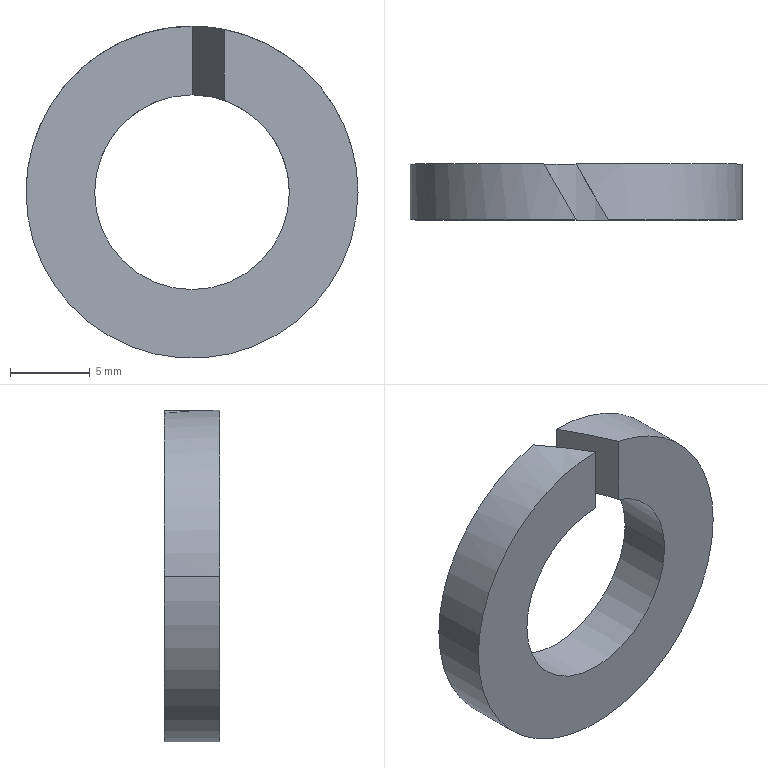Part | SolidWorks | features BaseBody 1 | 1 solid | 10 faces | box 20.8 x 3.5 x 20.8 mm | volume 749.557 mm3 | cylinder 6 | plane 4 | commonest cylinder face diameters 12.2 x3 20.8 x3
STEP:
#1=CARTESIAN_POINT('',(215.5,175.2,30.35));
#2=VERTEX_POINT('',#1);
#3=CARTESIAN_POINT('',(209.4,175.2,24.25));
#4=VERTEX_POINT('',#3);
#5=CARTESIAN_POINT('',(215.5,175.2,24.25));
#6=DIRECTION('',(0.,-1.,0.));
#7=DIRECTION('',(1.,0.,0.));
#8=AXIS2_PLACEMENT_3D('',#5,#6,#7);
#9=CIRCLE('',#8,6.1);
#10=EDGE_CURVE('',#2,#4,#9,.T.);
#11=ORIENTED_EDGE('',*,*,#10,.T.);
#12=CARTESIAN_POINT('',(209.4,178.7,24.25));
#13=VERTEX_POINT('',#12);
#14=CARTESIAN_POINT('',(209.4,175.2,24.25));
#15=DIRECTION('',(0.,1.,0.));
#16=VECTOR('',#15,1000.);
#17=LINE('',#14,#16);
#18=EDGE_CURVE('',#4,#13,#17,.T.);
#19=ORIENTED_EDGE('',*,*,#18,.T.);
#20=CARTESIAN_POINT('',(213.479,178.7,30.006));
#21=VERTEX_POINT('',#20);
#22=CARTESIAN_POINT('',(215.5,178.7,24.25));
#23=DIRECTION('',(0.,-1.,0.));
#24=DIRECTION('',(-1.,0.,0.));
#25=AXIS2_PLACEMENT_3D('',#22,#23,#24);
#26=CIRCLE('',#25,6.1);
#27=EDGE_CURVE('',#21,#13,#26,.T.);
#28=ORIENTED_EDGE('',*,*,#27,.F.);
#29=CARTESIAN_POINT('',(215.5,175.2,30.35));
#30=CARTESIAN_POINT('',(214.81,176.395,30.35));
#31=CARTESIAN_POINT('',(214.13,177.573,30.234));
#32=CARTESIAN_POINT('',(213.479,178.7,30.006));
#33=(BOUNDED_CURVE()B_SPLINE_CURVE(3,(#29,#30,#31,#32),.UNSPECIFIED.,.F.,.F.)B_SPLINE_CURVE_WITH_KNOTS((4,4),(4.712,5.05),.UNSPECIFIED.)CURVE()GEOMETRIC_REPRESENTATION_ITEM()RATIONAL_B_SPLINE_CURVE((1.,0.9905,0.9905,1.))REPRESENTATION_ITEM(''));
#34=EDGE_CURVE('',#2,#21,#33,.T.);
#35=ORIENTED_EDGE('',*,*,#34,.F.);
#36=EDGE_LOOP('',(#11,#19,#28,#35));
#37=FACE_OUTER_BOUND('',#36,.T.);
#38=CARTESIAN_POINT('',(215.5,175.2,24.25));
#39=DIRECTION('',(0.,1.,0.));
#40=DIRECTION('',(1.,0.,0.));
#41=AXIS2_PLACEMENT_3D('',#38,#39,#40);
#42=CYLINDRICAL_SURFACE('',#41,6.1);
#43=ADVANCED_FACE('',(#37),#42,.F.);
#44=ORIENTED_EDGE('',*,*,#18,.F.);
#45=CARTESIAN_POINT('',(221.6,175.2,24.25));
#46=VERTEX_POINT('',#45);
#47=CARTESIAN_POINT('',(215.5,175.2,24.25));
#48=DIRECTION('',(0.,-1.,0.));
#49=DIRECTION('',(1.,0.,0.));
#50=AXIS2_PLACEMENT_3D('',#47,#48,#49);
#51=CIRCLE('',#50,6.1);
#52=EDGE_CURVE('',#4,#46,#51,.T.);
#53=ORIENTED_EDGE('',*,*,#52,.T.);
#54=CARTESIAN_POINT('',(221.6,178.7,24.25));
#55=VERTEX_POINT('',#54);
#56=CARTESIAN_POINT('',(221.6,175.2,24.25));
#57=DIRECTION('',(0.,1.,0.));
#58=VECTOR('',#57,1000.);
#59=LINE('',#56,#58);
#60=EDGE_CURVE('',#46,#55,#59,.T.);
#61=ORIENTED_EDGE('',*,*,#60,.T.);
#62=CARTESIAN_POINT('',(215.5,178.7,24.25));
#63=DIRECTION('',(0.,-1.,0.));
#64=DIRECTION('',(-1.,0.,0.));
#65=AXIS2_PLACEMENT_3D('',#62,#63,#64);
#66=CIRCLE('',#65,6.1);
#67=EDGE_CURVE('',#13,#55,#66,.T.);
#68=ORIENTED_EDGE('',*,*,#67,.F.);
#69=EDGE_LOOP('',(#44,#53,#61,#68));
#70=FACE_OUTER_BOUND('',#69,.T.);
#71=CARTESIAN_POINT('',(215.5,175.2,24.25));
#72=DIRECTION('',(0.,1.,0.));
#73=DIRECTION('',(1.,0.,0.));
#74=AXIS2_PLACEMENT_3D('',#71,#72,#73);
#75=CYLINDRICAL_SURFACE('',#74,6.1);
#76=ADVANCED_FACE('',(#70),#75,.F.);
#77=CARTESIAN_POINT('',(205.1,175.2,24.25));
#78=VERTEX_POINT('',#77);
#79=CARTESIAN_POINT('',(225.9,175.2,24.25));
#80=VERTEX_POINT('',#79);
#81=CARTESIAN_POINT('',(215.5,175.2,24.25));
#82=DIRECTION('',(0.,-1.,0.));
#83=DIRECTION('',(1.,0.,0.));
#84=AXIS2_PLACEMENT_3D('',#81,#82,#83);
#85=CIRCLE('',#84,10.4);
#86=EDGE_CURVE('',#78,#80,#85,.T.);
#87=ORIENTED_EDGE('',*,*,#86,.F.);
#88=CARTESIAN_POINT('',(205.1,178.7,24.25));
#89=VERTEX_POINT('',#88);
#90=CARTESIAN_POINT('',(205.1,175.2,24.25));
#91=DIRECTION('',(0.,1.,0.));
#92=VECTOR('',#91,1000.);
#93=LINE('',#90,#92);
#94=EDGE_CURVE('',#78,#89,#93,.T.);
#95=ORIENTED_EDGE('',*,*,#94,.T.);
#96=CARTESIAN_POINT('',(225.9,178.7,24.25));
#97=VERTEX_POINT('',#96);
#98=CARTESIAN_POINT('',(215.5,178.7,24.25));
#99=DIRECTION('',(0.,-1.,0.));
#100=DIRECTION('',(-1.,0.,0.));
#101=AXIS2_PLACEMENT_3D('',#98,#99,#100);
#102=CIRCLE('',#101,10.4);
#103=EDGE_CURVE('',#89,#97,#102,.T.);
#104=ORIENTED_EDGE('',*,*,#103,.T.);
#105=CARTESIAN_POINT('',(225.9,175.2,24.25));
#106=DIRECTION('',(0.,1.,0.));
#107=VECTOR('',#106,1000.);
#108=LINE('',#105,#107);
#109=EDGE_CURVE('',#80,#97,#108,.T.);
#110=ORIENTED_EDGE('',*,*,#109,.F.);
#111=EDGE_LOOP('',(#87,#95,#104,#110));
#112=FACE_OUTER_BOUND('',#111,.T.);
#113=CARTESIAN_POINT('',(215.5,175.2,24.25));
#114=DIRECTION('',(0.,1.,0.));
#115=DIRECTION('',(1.,0.,0.));
#116=AXIS2_PLACEMENT_3D('',#113,#114,#115);
#117=CYLINDRICAL_SURFACE('',#116,10.4);
#118=ADVANCED_FACE('',(#112),#117,.T.);
#119=CARTESIAN_POINT('',(217.521,175.2,34.452));
#120=VERTEX_POINT('',#119);
#121=CARTESIAN_POINT('',(215.5,175.2,24.25));
#122=DIRECTION('',(0.,-1.,0.));
#123=DIRECTION('',(1.,0.,0.));
#124=AXIS2_PLACEMENT_3D('',#121,#122,#123);
#125=CIRCLE('',#124,10.4);
#126=EDGE_CURVE('',#80,#120,#125,.T.);
#127=ORIENTED_EDGE('',*,*,#126,.F.);
#128=ORIENTED_EDGE('',*,*,#109,.T.);
#129=CARTESIAN_POINT('',(215.5,178.7,34.65));
#130=VERTEX_POINT('',#129);
#131=CARTESIAN_POINT('',(215.5,178.7,24.25));
#132=DIRECTION('',(0.,-1.,0.));
#133=DIRECTION('',(-1.,0.,0.));
#134=AXIS2_PLACEMENT_3D('',#131,#132,#133);
#135=CIRCLE('',#134,10.4);
#136=EDGE_CURVE('',#97,#130,#135,.T.);
#137=ORIENTED_EDGE('',*,*,#136,.T.);
#138=CARTESIAN_POINT('',(215.5,178.7,34.65));
#139=CARTESIAN_POINT('',(216.179,177.524,34.65));
#140=CARTESIAN_POINT('',(216.855,176.354,34.584));
#141=CARTESIAN_POINT('',(217.521,175.2,34.452));
#142=(BOUNDED_CURVE()B_SPLINE_CURVE(3,(#138,#139,#140,#141),.UNSPECIFIED.,.F.,.F.)B_SPLINE_CURVE_WITH_KNOTS((4,4),(1.571,1.766),.UNSPECIFIED.)CURVE()GEOMETRIC_REPRESENTATION_ITEM()RATIONAL_B_SPLINE_CURVE((1.,0.9968,0.9968,1.))REPRESENTATION_ITEM(''));
#143=EDGE_CURVE('',#130,#120,#142,.T.);
#144=ORIENTED_EDGE('',*,*,#143,.T.);
#145=EDGE_LOOP('',(#127,#128,#137,#144));
#146=FACE_OUTER_BOUND('',#145,.T.);
#147=CARTESIAN_POINT('',(215.5,175.2,24.25));
#148=DIRECTION('',(0.,1.,0.));
#149=DIRECTION('',(1.,0.,0.));
#150=AXIS2_PLACEMENT_3D('',#147,#148,#149);
#151=CYLINDRICAL_SURFACE('',#150,10.4);
#152=ADVANCED_FACE('',(#146),#151,.T.);
#153=ORIENTED_EDGE('',*,*,#10,.F.);
#154=CARTESIAN_POINT('',(215.5,175.2,34.65));
#155=VERTEX_POINT('',#154);
#156=CARTESIAN_POINT('',(215.5,175.2,34.65));
#157=DIRECTION('',(0.,0.,-1.));
#158=VECTOR('',#157,1000.);
#159=LINE('',#156,#158);
#160=EDGE_CURVE('',#155,#2,#159,.T.);
#161=ORIENTED_EDGE('',*,*,#160,.F.);
#162=CARTESIAN_POINT('',(215.5,175.2,24.25));
#163=DIRECTION('',(0.,-1.,0.));
#164=DIRECTION('',(1.,0.,0.));
#165=AXIS2_PLACEMENT_3D('',#162,#163,#164);
#166=CIRCLE('',#165,10.4);
#167=EDGE_CURVE('',#155,#78,#166,.T.);
#168=ORIENTED_EDGE('',*,*,#167,.T.);
#169=ORIENTED_EDGE('',*,*,#86,.T.);
#170=ORIENTED_EDGE('',*,*,#126,.T.);
#171=CARTESIAN_POINT('',(217.521,175.2,30.006));
#172=VERTEX_POINT('',#171);
#173=CARTESIAN_POINT('',(217.521,175.2,34.65));
#174=DIRECTION('',(0.,0.,-1.));
#175=VECTOR('',#174,1000.);
#176=LINE('',#173,#175);
#177=EDGE_CURVE('',#120,#172,#176,.T.);
#178=ORIENTED_EDGE('',*,*,#177,.T.);
#179=CARTESIAN_POINT('',(215.5,175.2,24.25));
#180=DIRECTION('',(0.,-1.,0.));
#181=DIRECTION('',(1.,0.,0.));
#182=AXIS2_PLACEMENT_3D('',#179,#180,#181);
#183=CIRCLE('',#182,6.1);
#184=EDGE_CURVE('',#46,#172,#183,.T.);
#185=ORIENTED_EDGE('',*,*,#184,.F.);
#186=ORIENTED_EDGE('',*,*,#52,.F.);
#187=EDGE_LOOP('',(#153,#161,#168,#169,#170,#178,#185,#186));
#188=FACE_OUTER_BOUND('',#187,.T.);
#189=CARTESIAN_POINT('',(215.5,175.2,24.25));
#190=DIRECTION('',(0.,1.,0.));
#191=DIRECTION('',(1.,0.,0.));
#192=AXIS2_PLACEMENT_3D('',#189,#190,#191);
#193=PLANE('',#192);
#194=ADVANCED_FACE('',(#188),#193,.F.);
#195=CARTESIAN_POINT('',(213.479,178.7,34.452));
#196=VERTEX_POINT('',#195);
#197=CARTESIAN_POINT('',(213.479,178.7,34.65));
#198=DIRECTION('',(0.,0.,-1.));
#199=VECTOR('',#198,1000.);
#200=LINE('',#197,#199);
#201=EDGE_CURVE('',#196,#21,#200,.T.);
#202=ORIENTED_EDGE('',*,*,#201,.T.);
#203=ORIENTED_EDGE('',*,*,#27,.T.);
#204=ORIENTED_EDGE('',*,*,#67,.T.);
#205=CARTESIAN_POINT('',(215.5,178.7,30.35));
#206=VERTEX_POINT('',#205);
#207=CARTESIAN_POINT('',(215.5,178.7,24.25));
#208=DIRECTION('',(0.,-1.,0.));
#209=DIRECTION('',(-1.,0.,0.));
#210=AXIS2_PLACEMENT_3D('',#207,#208,#209);
#211=CIRCLE('',#210,6.1);
#212=EDGE_CURVE('',#55,#206,#211,.T.);
#213=ORIENTED_EDGE('',*,*,#212,.T.);
#214=CARTESIAN_POINT('',(215.5,178.7,34.65));
#215=DIRECTION('',(0.,0.,-1.));
#216=VECTOR('',#215,1000.);
#217=LINE('',#214,#216);
#218=EDGE_CURVE('',#130,#206,#217,.T.);
#219=ORIENTED_EDGE('',*,*,#218,.F.);
#220=ORIENTED_EDGE('',*,*,#136,.F.);
#221=ORIENTED_EDGE('',*,*,#103,.F.);
#222=CARTESIAN_POINT('',(215.5,178.7,24.25));
#223=DIRECTION('',(0.,-1.,0.));
#224=DIRECTION('',(-1.,0.,0.));
#225=AXIS2_PLACEMENT_3D('',#222,#223,#224);
#226=CIRCLE('',#225,10.4);
#227=EDGE_CURVE('',#196,#89,#226,.T.);
#228=ORIENTED_EDGE('',*,*,#227,.F.);
#229=EDGE_LOOP('',(#202,#203,#204,#213,#219,#220,#221,#228));
#230=FACE_OUTER_BOUND('',#229,.T.);
#231=CARTESIAN_POINT('',(215.5,178.7,24.25));
#232=DIRECTION('',(0.,1.,0.));
#233=DIRECTION('',(1.,0.,0.));
#234=AXIS2_PLACEMENT_3D('',#231,#232,#233);
#235=PLANE('',#234);
#236=ADVANCED_FACE('',(#230),#235,.T.);
#237=ORIENTED_EDGE('',*,*,#94,.F.);
#238=ORIENTED_EDGE('',*,*,#167,.F.);
#239=CARTESIAN_POINT('',(215.5,175.2,34.65));
#240=CARTESIAN_POINT('',(214.821,176.376,34.65));
#241=CARTESIAN_POINT('',(214.145,177.546,34.584));
#242=CARTESIAN_POINT('',(213.479,178.7,34.452));
#243=(BOUNDED_CURVE()B_SPLINE_CURVE(3,(#239,#240,#241,#242),.UNSPECIFIED.,.F.,.F.)B_SPLINE_CURVE_WITH_KNOTS((4,4),(4.712,4.908),.UNSPECIFIED.)CURVE()GEOMETRIC_REPRESENTATION_ITEM()RATIONAL_B_SPLINE_CURVE((1.,0.9968,0.9968,1.))REPRESENTATION_ITEM(''));
#244=EDGE_CURVE('',#155,#196,#243,.T.);
#245=ORIENTED_EDGE('',*,*,#244,.T.);
#246=ORIENTED_EDGE('',*,*,#227,.T.);
#247=EDGE_LOOP('',(#237,#238,#245,#246));
#248=FACE_OUTER_BOUND('',#247,.T.);
#249=CARTESIAN_POINT('',(215.5,175.2,24.25));
#250=DIRECTION('',(0.,1.,0.));
#251=DIRECTION('',(1.,0.,0.));
#252=AXIS2_PLACEMENT_3D('',#249,#250,#251);
#253=CYLINDRICAL_SURFACE('',#252,10.4);
#254=ADVANCED_FACE('',(#248),#253,.T.);
#255=ORIENTED_EDGE('',*,*,#60,.F.);
#256=ORIENTED_EDGE('',*,*,#184,.T.);
#257=CARTESIAN_POINT('',(215.5,178.7,30.35));
#258=CARTESIAN_POINT('',(216.19,177.505,30.35));
#259=CARTESIAN_POINT('',(216.87,176.327,30.234));
#260=CARTESIAN_POINT('',(217.521,175.2,30.006));
#261=(BOUNDED_CURVE()B_SPLINE_CURVE(3,(#257,#258,#259,#260),.UNSPECIFIED.,.F.,.F.)B_SPLINE_CURVE_WITH_KNOTS((4,4),(1.571,1.908),.UNSPECIFIED.)CURVE()GEOMETRIC_REPRESENTATION_ITEM()RATIONAL_B_SPLINE_CURVE((1.,0.9905,0.9905,1.))REPRESENTATION_ITEM(''));
#262=EDGE_CURVE('',#206,#172,#261,.T.);
#263=ORIENTED_EDGE('',*,*,#262,.F.);
#264=ORIENTED_EDGE('',*,*,#212,.F.);
#265=EDGE_LOOP('',(#255,#256,#263,#264));
#266=FACE_OUTER_BOUND('',#265,.T.);
#267=CARTESIAN_POINT('',(215.5,175.2,24.25));
#268=DIRECTION('',(0.,1.,0.));
#269=DIRECTION('',(1.,0.,0.));
#270=AXIS2_PLACEMENT_3D('',#267,#268,#269);
#271=CYLINDRICAL_SURFACE('',#270,6.1);
#272=ADVANCED_FACE('',(#266),#271,.F.);
#273=ORIENTED_EDGE('',*,*,#218,.T.);
#274=ORIENTED_EDGE('',*,*,#262,.T.);
#275=ORIENTED_EDGE('',*,*,#177,.F.);
#276=ORIENTED_EDGE('',*,*,#143,.F.);
#277=EDGE_LOOP('',(#273,#274,#275,#276));
#278=FACE_OUTER_BOUND('',#277,.T.);
#279=CARTESIAN_POINT('',(217.521,175.2,34.65));
#280=DIRECTION('',(0.866,0.5,0.));
#281=DIRECTION('',(0.5,-0.866,0.));
#282=AXIS2_PLACEMENT_3D('',#279,#280,#281);
#283=PLANE('',#282);
#284=ADVANCED_FACE('',(#278),#283,.F.);
#285=ORIENTED_EDGE('',*,*,#160,.T.);
#286=ORIENTED_EDGE('',*,*,#34,.T.);
#287=ORIENTED_EDGE('',*,*,#201,.F.);
#288=ORIENTED_EDGE('',*,*,#244,.F.);
#289=EDGE_LOOP('',(#285,#286,#287,#288));
#290=FACE_OUTER_BOUND('',#289,.T.);
#291=CARTESIAN_POINT('',(213.479,178.7,34.65));
#292=DIRECTION('',(-0.866,-0.5,0.));
#293=DIRECTION('',(-0.5,0.866,0.));
#294=AXIS2_PLACEMENT_3D('',#291,#292,#293);
#295=PLANE('',#294);
#296=ADVANCED_FACE('',(#290),#295,.F.);
#297=CLOSED_SHELL('',(#43,#76,#118,#152,#194,#236,#254,#272,#284,#296));
#298=MANIFOLD_SOLID_BREP('',#297);
#299=CARTESIAN_POINT('',(0.,0.,0.));
#300=DIRECTION('',(0.,0.,1.));
#301=DIRECTION('',(1.,0.,0.));
#302=AXIS2_PLACEMENT_3D('',#299,#300,#301);
#303=(LENGTH_UNIT()NAMED_UNIT(*)SI_UNIT(.MILLI.,.METRE.));
#304=UNCERTAINTY_MEASURE_WITH_UNIT(LENGTH_MEASURE(0.00001),#303,'','');
#305=(NAMED_UNIT(*)PLANE_ANGLE_UNIT()SI_UNIT($,.RADIAN.));
#306=(NAMED_UNIT(*)SI_UNIT($,.STERADIAN.)SOLID_ANGLE_UNIT());
#307=(GEOMETRIC_REPRESENTATION_CONTEXT(3)GLOBAL_UNCERTAINTY_ASSIGNED_CONTEXT((#304))GLOBAL_UNIT_ASSIGNED_CONTEXT((#303,#305,#306))REPRESENTATION_CONTEXT('',''));
#308=ADVANCED_BREP_SHAPE_REPRESENTATION('',(#298,#302),#307);